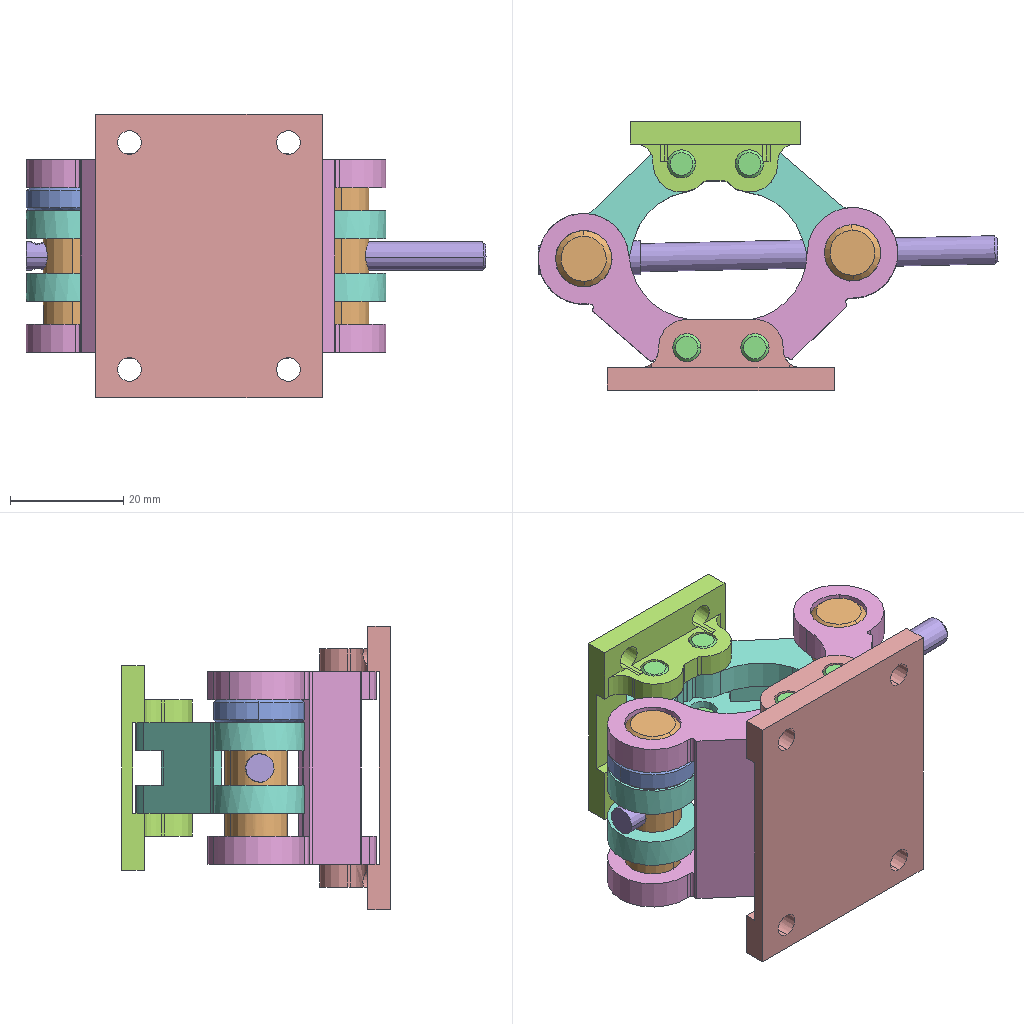Assembly | SolidWorks | 8 different items | 18 placed | box 81 x 47 x 50 mm
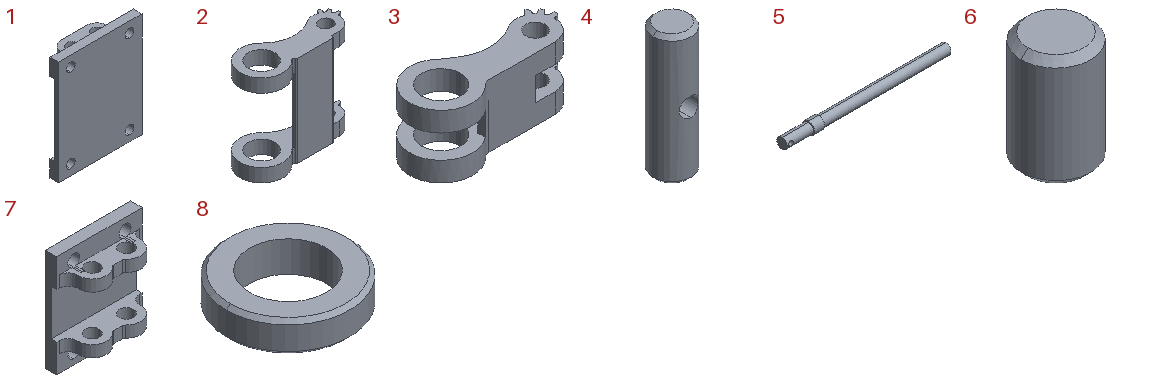Parts list (item | quantity | size | volume | features):
1 | x1 | 40 x 12.5 x 50 mm | 6181 mm3 | features HoleWzd 3, ICE 3, Fillet 2, Extrusion 1
2 | x2 | 38.562 x 16 x 34 mm | 4236 mm3 | features HoleWzd 4, ICE 4, Fillet 2, RefSurface 2, ThickenCut 2, Extrusion 1
3 | x2 | 38.582 x 16 x 16 mm | 3069 mm3 | features HoleWzd 4, ICE 4, Fillet 2, RefSurface 2, ThickenCut 2, Extrusion 1
4 | x2 | 10 x 10 x 34 mm | 2451 mm3 | features 3DProfileFeature 1, Chamfer 1, HoleWzd 1, Revolution 1
5 | x1 | 81 x 6 x 6 mm | 1608 mm3 | features ICE 2, 3DProfileFeature 1, Chamfer 1, HoleWzd 1, Revolution 1
6 | x8 | 5 x 5 x 8 mm | 153.414 mm3 | features Revolution 1
7 | x1 | 30 x 12.5 x 36 mm | 4162 mm3 | features ICE 12, RevCut 4, Fillet 2, HoleWzd 2, BaseBody 1
8 | x1 | 16 x 16 x 4 mm | 477.784 mm3 | features Revolution 1
Mates (type | each side: item.copy, entity, surface, feature):
Concentric | 1.1 face cylinder Ø5.0 (5) Diameter Hole1 | 2.1 face cylinder Ø5.0 (5) Diameter Hole1
Coincident | 1.1 face plane Cut-Extrude1 | 2.1 face plane Boss-Extrude3
Concentric | 2.1 face cylinder Ø10.0 (10) Diameter Hole1 | 4.1 face cylinder Revolve1
Coincident | 2.1 face plane Boss-Extrude3 | 4.1 face plane Revolve1
Coincident | 8.1 face plane Revolve1 | 2.1 face plane Boss-Extrude3
Concentric | 8.1 face cylinder Revolve1 | 4.1 face cylinder Revolve1
Concentric | 3.1 face cylinder Ø10.0 (10) Diameter Hole1 | 4.1 face cylinder Revolve1
Coincident | 8.1 face plane Revolve1 | 3.1 face plane Boss-Extrude1
Coincident | 7.1 face cylinder Ø5.0 (5) Diameter Hole2 | 3.1 edge
Coincident | 7.1 face plane Cut-Extrude1 | 3.1 face plane Boss-Extrude1
Concentric | 7.1 face cylinder Ø5.0 (5) Diameter Hole2 | 6.1 face cylinder Revolve1
Coincident | 7.1 face plane Input3 | 6.1 face plane Revolve1
Concentric | 4.1 face cylinder Ø5.0 (5) Diameter Hole1 | 5.1 face cylinder Boss-Extrude1
Tangent | 4.1 face cylinder Revolve1 | 5.1 face plane Revolve1
Concentric | 7.1 face cylinder Ø5.0 (5) Diameter Hole2 | 3.2 face cylinder Ø5.0 (5) Diameter Hole2
Coincident | 7.1 face plane Cut-Extrude1 | 3.2 face plane Boss-Extrude3
Concentric | 2.2 face cylinder Ø10.0 (10) Diameter Hole2 | 3.2 face cylinder Ø10.0 (10) Diameter Hole2
Concentric | 1.1 face cylinder Ø5.0 (5) Diameter Hole1 | 2.2 face cylinder Ø5.0 (5) Diameter Hole2
Coincident | 1.1 edge | 2.2 face plane Boss-Extrude1
Concentric | 5.1 face cylinder Boss-Extrude2 | 4.2 face cylinder Ø5.0 (5) Diameter Hole1
Concentric | 4.2 face cylinder Revolve1 | 2.2 face cylinder Ø10.0 (10) Diameter Hole2
Parallel | 1.1 face plane Cut-Extrude1 | 7.1 face plane Boss-Extrude3
Concentric | 6.2 face cylinder Revolve1 | 2.2 face cylinder Ø5.0 (5) Diameter Hole1
Coincident | 6.2 face plane Revolve1 | 2.2 face plane Boss-Extrude3
Concentric | 2.1 face cylinder Ø5.0 (5) Diameter Hole2 | 6.3 face cylinder Revolve1
Coincident | 2.1 face plane Boss-Extrude1 | 6.3 face plane Revolve1
Concentric | 2.1 face cylinder Ø5.0 (5) Diameter Hole1 | 6.4 face cylinder Revolve1
Coincident | 1.1 face plane Boss-Extrude3 | 6.4 face plane Revolve1
Concentric | 1.1 face cylinder Ø5.0 (5) Diameter Hole1 | 6.5 face cylinder Revolve1
Coincident | 1.1 face plane Boss-Extrude3 | 6.5 face plane Revolve1
Concentric | 7.1 face cylinder Ø5.0 (5) Diameter Hole2 | 6.6 face cylinder Revolve1
Coincident | 7.1 face plane Input3 | 6.6 face plane Revolve1
Concentric | 7.1 face cylinder Ø5.0 (5) Diameter Hole1 | 6.7 face cylinder Revolve1
Coincident | 7.1 face plane Input3 | 6.7 face plane Revolve1
Concentric | 7.1 face cylinder Ø5.0 (5) Diameter Hole1 | 6.8 face cylinder Revolve1
Coincident | 7.1 face plane Input3 | 6.8 face plane Revolve1